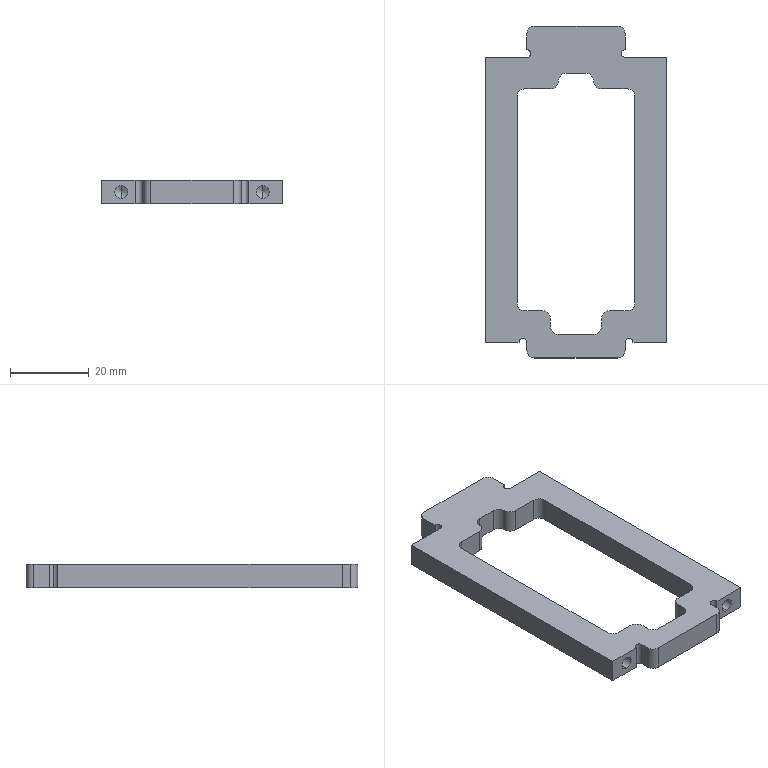Part | SolidWorks | features Fillet 2, HoleWzd 2, ICE 2, Extrusion 1 | 1 solid | 61 faces | box 46 x 84.45 x 6 mm | volume 10492 mm3 | cylinder 29 | plane 24 | cone 8 | commonest cylinder face diameters 4 x16 3.3 x8 2 x5